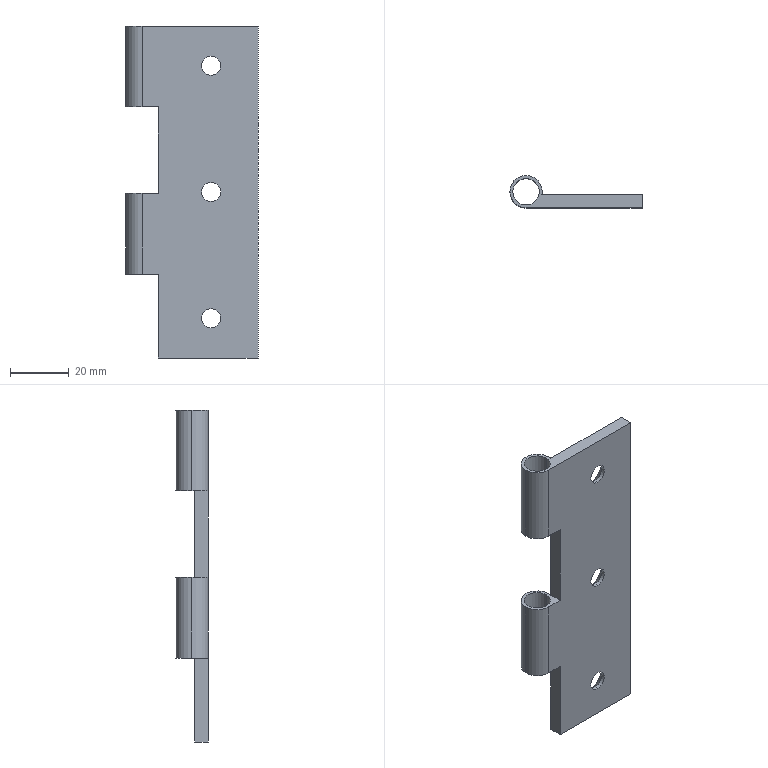Part | SolidWorks | features BaseBody 1 | 1 solid | 32 faces | box 45 x 11 x 113 mm | volume 18493 mm3 | cylinder 16 | plane 10 | cone 6 | commonest cylinder face diameters 6.5 x6 11 x6 9 x4
STEP:
#1=CARTESIAN_POINT('',(23.5,0.,3.25));
#2=VERTEX_POINT('',#1);
#3=CARTESIAN_POINT('',(23.5,0.,-3.25));
#4=VERTEX_POINT('',#3);
#5=CARTESIAN_POINT('',(23.5,0.,0.));
#6=DIRECTION('',(0.,-1.,0.));
#7=DIRECTION('',(0.,0.,1.));
#8=AXIS2_PLACEMENT_3D('',#5,#6,#7);
#9=CIRCLE('',#8,3.25);
#10=EDGE_CURVE('',#2,#4,#9,.T.);
#11=ORIENTED_EDGE('',*,*,#10,.T.);
#12=CARTESIAN_POINT('',(23.5,1.25,-3.25));
#13=VERTEX_POINT('',#12);
#14=CARTESIAN_POINT('',(23.5,0.,-3.25));
#15=DIRECTION('',(0.,1.,0.));
#16=VECTOR('',#15,1000.);
#17=LINE('',#14,#16);
#18=EDGE_CURVE('',#4,#13,#17,.T.);
#19=ORIENTED_EDGE('',*,*,#18,.T.);
#20=CARTESIAN_POINT('',(23.5,1.25,3.25));
#21=VERTEX_POINT('',#20);
#22=CARTESIAN_POINT('',(23.5,1.25,0.));
#23=DIRECTION('',(0.,-1.,0.));
#24=DIRECTION('',(0.,0.,1.));
#25=AXIS2_PLACEMENT_3D('',#22,#23,#24);
#26=CIRCLE('',#25,3.25);
#27=EDGE_CURVE('',#21,#13,#26,.T.);
#28=ORIENTED_EDGE('',*,*,#27,.F.);
#29=CARTESIAN_POINT('',(23.5,0.,3.25));
#30=DIRECTION('',(0.,1.,0.));
#31=VECTOR('',#30,1000.);
#32=LINE('',#29,#31);
#33=EDGE_CURVE('',#2,#21,#32,.T.);
#34=ORIENTED_EDGE('',*,*,#33,.F.);
#35=EDGE_LOOP('',(#11,#19,#28,#34));
#36=FACE_OUTER_BOUND('',#35,.T.);
#37=CARTESIAN_POINT('',(23.5,0.,0.));
#38=DIRECTION('',(0.,1.,0.));
#39=DIRECTION('',(0.,0.,1.));
#40=AXIS2_PLACEMENT_3D('',#37,#38,#39);
#41=CYLINDRICAL_SURFACE('',#40,3.25);
#42=ADVANCED_FACE('',(#36),#41,.F.);
#43=CARTESIAN_POINT('',(23.5,0.,46.25));
#44=VERTEX_POINT('',#43);
#45=CARTESIAN_POINT('',(23.5,0.,39.75));
#46=VERTEX_POINT('',#45);
#47=CARTESIAN_POINT('',(23.5,0.,43.));
#48=DIRECTION('',(0.,-1.,0.));
#49=DIRECTION('',(0.,0.,1.));
#50=AXIS2_PLACEMENT_3D('',#47,#48,#49);
#51=CIRCLE('',#50,3.25);
#52=EDGE_CURVE('',#44,#46,#51,.T.);
#53=ORIENTED_EDGE('',*,*,#52,.T.);
#54=CARTESIAN_POINT('',(23.5,1.25,39.75));
#55=VERTEX_POINT('',#54);
#56=CARTESIAN_POINT('',(23.5,0.,39.75));
#57=DIRECTION('',(0.,1.,0.));
#58=VECTOR('',#57,1000.);
#59=LINE('',#56,#58);
#60=EDGE_CURVE('',#46,#55,#59,.T.);
#61=ORIENTED_EDGE('',*,*,#60,.T.);
#62=CARTESIAN_POINT('',(23.5,1.25,46.25));
#63=VERTEX_POINT('',#62);
#64=CARTESIAN_POINT('',(23.5,1.25,43.));
#65=DIRECTION('',(0.,-1.,0.));
#66=DIRECTION('',(0.,0.,1.));
#67=AXIS2_PLACEMENT_3D('',#64,#65,#66);
#68=CIRCLE('',#67,3.25);
#69=EDGE_CURVE('',#63,#55,#68,.T.);
#70=ORIENTED_EDGE('',*,*,#69,.F.);
#71=CARTESIAN_POINT('',(23.5,0.,46.25));
#72=DIRECTION('',(0.,1.,0.));
#73=VECTOR('',#72,1000.);
#74=LINE('',#71,#73);
#75=EDGE_CURVE('',#44,#63,#74,.T.);
#76=ORIENTED_EDGE('',*,*,#75,.F.);
#77=EDGE_LOOP('',(#53,#61,#70,#76));
#78=FACE_OUTER_BOUND('',#77,.T.);
#79=CARTESIAN_POINT('',(23.5,0.,43.));
#80=DIRECTION('',(0.,1.,0.));
#81=DIRECTION('',(0.,0.,1.));
#82=AXIS2_PLACEMENT_3D('',#79,#80,#81);
#83=CYLINDRICAL_SURFACE('',#82,3.25);
#84=ADVANCED_FACE('',(#78),#83,.F.);
#85=CARTESIAN_POINT('',(23.5,0.,-39.75));
#86=VERTEX_POINT('',#85);
#87=CARTESIAN_POINT('',(23.5,0.,-46.25));
#88=VERTEX_POINT('',#87);
#89=CARTESIAN_POINT('',(23.5,0.,-43.));
#90=DIRECTION('',(0.,-1.,0.));
#91=DIRECTION('',(0.,0.,1.));
#92=AXIS2_PLACEMENT_3D('',#89,#90,#91);
#93=CIRCLE('',#92,3.25);
#94=EDGE_CURVE('',#86,#88,#93,.T.);
#95=ORIENTED_EDGE('',*,*,#94,.T.);
#96=CARTESIAN_POINT('',(23.5,1.25,-46.25));
#97=VERTEX_POINT('',#96);
#98=CARTESIAN_POINT('',(23.5,0.,-46.25));
#99=DIRECTION('',(0.,1.,0.));
#100=VECTOR('',#99,1000.);
#101=LINE('',#98,#100);
#102=EDGE_CURVE('',#88,#97,#101,.T.);
#103=ORIENTED_EDGE('',*,*,#102,.T.);
#104=CARTESIAN_POINT('',(23.5,1.25,-39.75));
#105=VERTEX_POINT('',#104);
#106=CARTESIAN_POINT('',(23.5,1.25,-43.));
#107=DIRECTION('',(0.,-1.,0.));
#108=DIRECTION('',(0.,0.,1.));
#109=AXIS2_PLACEMENT_3D('',#106,#107,#108);
#110=CIRCLE('',#109,3.25);
#111=EDGE_CURVE('',#105,#97,#110,.T.);
#112=ORIENTED_EDGE('',*,*,#111,.F.);
#113=CARTESIAN_POINT('',(23.5,0.,-39.75));
#114=DIRECTION('',(0.,1.,0.));
#115=VECTOR('',#114,1000.);
#116=LINE('',#113,#115);
#117=EDGE_CURVE('',#86,#105,#116,.T.);
#118=ORIENTED_EDGE('',*,*,#117,.F.);
#119=EDGE_LOOP('',(#95,#103,#112,#118));
#120=FACE_OUTER_BOUND('',#119,.T.);
#121=CARTESIAN_POINT('',(23.5,0.,-43.));
#122=DIRECTION('',(0.,1.,0.));
#123=DIRECTION('',(0.,0.,1.));
#124=AXIS2_PLACEMENT_3D('',#121,#122,#123);
#125=CYLINDRICAL_SURFACE('',#124,3.25);
#126=ADVANCED_FACE('',(#120),#125,.F.);
#127=CARTESIAN_POINT('',(5.5,5.5,-28.));
#128=VERTEX_POINT('',#127);
#129=CARTESIAN_POINT('',(-5.5,5.5,-28.));
#130=VERTEX_POINT('',#129);
#131=CARTESIAN_POINT('',(0.,5.5,-28.));
#132=DIRECTION('',(0.,0.,1.));
#133=DIRECTION('',(1.,0.,0.));
#134=AXIS2_PLACEMENT_3D('',#131,#132,#133);
#135=CIRCLE('',#134,5.5);
#136=EDGE_CURVE('',#128,#130,#135,.T.);
#137=ORIENTED_EDGE('',*,*,#136,.T.);
#138=CARTESIAN_POINT('',(-5.5,5.5,-0.5));
#139=VERTEX_POINT('',#138);
#140=CARTESIAN_POINT('',(-5.5,5.5,56.5));
#141=DIRECTION('',(0.,0.,1.));
#142=VECTOR('',#141,1000.);
#143=LINE('',#140,#142);
#144=EDGE_CURVE('',#130,#139,#143,.T.);
#145=ORIENTED_EDGE('',*,*,#144,.T.);
#146=CARTESIAN_POINT('',(5.5,5.5,-0.5));
#147=VERTEX_POINT('',#146);
#148=CARTESIAN_POINT('',(0.,5.5,-0.5));
#149=DIRECTION('',(0.,0.,1.));
#150=DIRECTION('',(1.,0.,0.));
#151=AXIS2_PLACEMENT_3D('',#148,#149,#150);
#152=CIRCLE('',#151,5.5);
#153=EDGE_CURVE('',#147,#139,#152,.T.);
#154=ORIENTED_EDGE('',*,*,#153,.F.);
#155=CARTESIAN_POINT('',(5.5,5.5,56.5));
#156=DIRECTION('',(0.,0.,1.));
#157=VECTOR('',#156,1000.);
#158=LINE('',#155,#157);
#159=EDGE_CURVE('',#128,#147,#158,.T.);
#160=ORIENTED_EDGE('',*,*,#159,.F.);
#161=EDGE_LOOP('',(#137,#145,#154,#160));
#162=FACE_OUTER_BOUND('',#161,.T.);
#163=CARTESIAN_POINT('',(0.,5.5,56.5));
#164=DIRECTION('',(0.,0.,1.));
#165=DIRECTION('',(1.,0.,0.));
#166=AXIS2_PLACEMENT_3D('',#163,#164,#165);
#167=CYLINDRICAL_SURFACE('',#166,5.5);
#168=ADVANCED_FACE('',(#162),#167,.T.);
#169=CARTESIAN_POINT('',(5.408,4.5,-28.));
#170=VERTEX_POINT('',#169);
#171=CARTESIAN_POINT('',(0.,5.5,-28.));
#172=DIRECTION('',(0.,0.,1.));
#173=DIRECTION('',(1.,0.,0.));
#174=AXIS2_PLACEMENT_3D('',#171,#172,#173);
#175=CIRCLE('',#174,5.5);
#176=EDGE_CURVE('',#170,#128,#175,.T.);
#177=ORIENTED_EDGE('',*,*,#176,.T.);
#178=ORIENTED_EDGE('',*,*,#159,.T.);
#179=CARTESIAN_POINT('',(5.408,4.5,-0.5));
#180=VERTEX_POINT('',#179);
#181=CARTESIAN_POINT('',(0.,5.5,-0.5));
#182=DIRECTION('',(0.,0.,1.));
#183=DIRECTION('',(1.,0.,0.));
#184=AXIS2_PLACEMENT_3D('',#181,#182,#183);
#185=CIRCLE('',#184,5.5);
#186=EDGE_CURVE('',#180,#147,#185,.T.);
#187=ORIENTED_EDGE('',*,*,#186,.F.);
#188=CARTESIAN_POINT('',(5.408,4.5,56.5));
#189=DIRECTION('',(0.,0.,-1.));
#190=VECTOR('',#189,1000.);
#191=LINE('',#188,#190);
#192=EDGE_CURVE('',#180,#170,#191,.T.);
#193=ORIENTED_EDGE('',*,*,#192,.T.);
#194=EDGE_LOOP('',(#177,#178,#187,#193));
#195=FACE_OUTER_BOUND('',#194,.T.);
#196=CARTESIAN_POINT('',(0.,5.5,56.5));
#197=DIRECTION('',(0.,0.,1.));
#198=DIRECTION('',(1.,0.,0.));
#199=AXIS2_PLACEMENT_3D('',#196,#197,#198);
#200=CYLINDRICAL_SURFACE('',#199,5.5);
#201=ADVANCED_FACE('',(#195),#200,.T.);
#202=CARTESIAN_POINT('',(5.5,5.5,29.));
#203=VERTEX_POINT('',#202);
#204=CARTESIAN_POINT('',(-5.5,5.5,29.));
#205=VERTEX_POINT('',#204);
#206=CARTESIAN_POINT('',(0.,5.5,29.));
#207=DIRECTION('',(0.,0.,1.));
#208=DIRECTION('',(1.,0.,0.));
#209=AXIS2_PLACEMENT_3D('',#206,#207,#208);
#210=CIRCLE('',#209,5.5);
#211=EDGE_CURVE('',#203,#205,#210,.T.);
#212=ORIENTED_EDGE('',*,*,#211,.T.);
#213=CARTESIAN_POINT('',(-5.5,5.5,56.5));
#214=VERTEX_POINT('',#213);
#215=CARTESIAN_POINT('',(-5.5,5.5,56.5));
#216=DIRECTION('',(0.,0.,1.));
#217=VECTOR('',#216,1000.);
#218=LINE('',#215,#217);
#219=EDGE_CURVE('',#205,#214,#218,.T.);
#220=ORIENTED_EDGE('',*,*,#219,.T.);
#221=CARTESIAN_POINT('',(5.5,5.5,56.5));
#222=VERTEX_POINT('',#221);
#223=CARTESIAN_POINT('',(0.,5.5,56.5));
#224=DIRECTION('',(0.,0.,1.));
#225=DIRECTION('',(1.,0.,0.));
#226=AXIS2_PLACEMENT_3D('',#223,#224,#225);
#227=CIRCLE('',#226,5.5);
#228=EDGE_CURVE('',#222,#214,#227,.T.);
#229=ORIENTED_EDGE('',*,*,#228,.F.);
#230=CARTESIAN_POINT('',(5.5,5.5,56.5));
#231=DIRECTION('',(0.,0.,1.));
#232=VECTOR('',#231,1000.);
#233=LINE('',#230,#232);
#234=EDGE_CURVE('',#203,#222,#233,.T.);
#235=ORIENTED_EDGE('',*,*,#234,.F.);
#236=EDGE_LOOP('',(#212,#220,#229,#235));
#237=FACE_OUTER_BOUND('',#236,.T.);
#238=CARTESIAN_POINT('',(0.,5.5,56.5));
#239=DIRECTION('',(0.,0.,1.));
#240=DIRECTION('',(1.,0.,0.));
#241=AXIS2_PLACEMENT_3D('',#238,#239,#240);
#242=CYLINDRICAL_SURFACE('',#241,5.5);
#243=ADVANCED_FACE('',(#237),#242,.T.);
#244=CARTESIAN_POINT('',(5.408,4.5,29.));
#245=VERTEX_POINT('',#244);
#246=CARTESIAN_POINT('',(0.,5.5,29.));
#247=DIRECTION('',(0.,0.,1.));
#248=DIRECTION('',(1.,0.,0.));
#249=AXIS2_PLACEMENT_3D('',#246,#247,#248);
#250=CIRCLE('',#249,5.5);
#251=EDGE_CURVE('',#245,#203,#250,.T.);
#252=ORIENTED_EDGE('',*,*,#251,.T.);
#253=ORIENTED_EDGE('',*,*,#234,.T.);
#254=CARTESIAN_POINT('',(5.408,4.5,56.5));
#255=VERTEX_POINT('',#254);
#256=CARTESIAN_POINT('',(0.,5.5,56.5));
#257=DIRECTION('',(0.,0.,1.));
#258=DIRECTION('',(1.,0.,0.));
#259=AXIS2_PLACEMENT_3D('',#256,#257,#258);
#260=CIRCLE('',#259,5.5);
#261=EDGE_CURVE('',#255,#222,#260,.T.);
#262=ORIENTED_EDGE('',*,*,#261,.F.);
#263=CARTESIAN_POINT('',(5.408,4.5,56.5));
#264=DIRECTION('',(0.,0.,-1.));
#265=VECTOR('',#264,1000.);
#266=LINE('',#263,#265);
#267=EDGE_CURVE('',#255,#245,#266,.T.);
#268=ORIENTED_EDGE('',*,*,#267,.T.);
#269=EDGE_LOOP('',(#252,#253,#262,#268));
#270=FACE_OUTER_BOUND('',#269,.T.);
#271=CARTESIAN_POINT('',(0.,5.5,56.5));
#272=DIRECTION('',(0.,0.,1.));
#273=DIRECTION('',(1.,0.,0.));
#274=AXIS2_PLACEMENT_3D('',#271,#272,#273);
#275=CYLINDRICAL_SURFACE('',#274,5.5);
#276=ADVANCED_FACE('',(#270),#275,.T.);
#277=ORIENTED_EDGE('',*,*,#27,.T.);
#278=CARTESIAN_POINT('',(23.5,4.5,-6.5));
#279=VERTEX_POINT('',#278);
#280=CARTESIAN_POINT('',(23.5,4.5,-6.5));
#281=DIRECTION('',(0.,0.7071,-0.7071));
#282=VECTOR('',#281,1000.);
#283=LINE('',#280,#282);
#284=EDGE_CURVE('',#13,#279,#283,.T.);
#285=ORIENTED_EDGE('',*,*,#284,.T.);
#286=CARTESIAN_POINT('',(23.5,4.5,6.5));
#287=VERTEX_POINT('',#286);
#288=CARTESIAN_POINT('',(23.5,4.5,0.));
#289=DIRECTION('',(0.,-1.,0.));
#290=DIRECTION('',(0.,0.,1.));
#291=AXIS2_PLACEMENT_3D('',#288,#289,#290);
#292=CIRCLE('',#291,6.5);
#293=EDGE_CURVE('',#287,#279,#292,.T.);
#294=ORIENTED_EDGE('',*,*,#293,.F.);
#295=CARTESIAN_POINT('',(23.5,4.5,6.5));
#296=DIRECTION('',(0.,0.7071,0.7071));
#297=VECTOR('',#296,1000.);
#298=LINE('',#295,#297);
#299=EDGE_CURVE('',#21,#287,#298,.T.);
#300=ORIENTED_EDGE('',*,*,#299,.F.);
#301=EDGE_LOOP('',(#277,#285,#294,#300));
#302=FACE_OUTER_BOUND('',#301,.T.);
#303=CARTESIAN_POINT('',(23.5,4.5,0.));
#304=DIRECTION('',(0.,1.,0.));
#305=DIRECTION('',(0.,0.,1.));
#306=AXIS2_PLACEMENT_3D('',#303,#304,#305);
#307=CONICAL_SURFACE('',#306,6.5,0.7854);
#308=ADVANCED_FACE('',(#302),#307,.F.);
#309=ORIENTED_EDGE('',*,*,#69,.T.);
#310=CARTESIAN_POINT('',(23.5,4.5,36.5));
#311=VERTEX_POINT('',#310);
#312=CARTESIAN_POINT('',(23.5,4.5,36.5));
#313=DIRECTION('',(0.,0.7071,-0.7071));
#314=VECTOR('',#313,1000.);
#315=LINE('',#312,#314);
#316=EDGE_CURVE('',#55,#311,#315,.T.);
#317=ORIENTED_EDGE('',*,*,#316,.T.);
#318=CARTESIAN_POINT('',(23.5,4.5,49.5));
#319=VERTEX_POINT('',#318);
#320=CARTESIAN_POINT('',(23.5,4.5,43.));
#321=DIRECTION('',(0.,-1.,0.));
#322=DIRECTION('',(0.,0.,1.));
#323=AXIS2_PLACEMENT_3D('',#320,#321,#322);
#324=CIRCLE('',#323,6.5);
#325=EDGE_CURVE('',#319,#311,#324,.T.);
#326=ORIENTED_EDGE('',*,*,#325,.F.);
#327=CARTESIAN_POINT('',(23.5,4.5,49.5));
#328=DIRECTION('',(0.,0.7071,0.7071));
#329=VECTOR('',#328,1000.);
#330=LINE('',#327,#329);
#331=EDGE_CURVE('',#63,#319,#330,.T.);
#332=ORIENTED_EDGE('',*,*,#331,.F.);
#333=EDGE_LOOP('',(#309,#317,#326,#332));
#334=FACE_OUTER_BOUND('',#333,.T.);
#335=CARTESIAN_POINT('',(23.5,4.5,43.));
#336=DIRECTION('',(0.,1.,0.));
#337=DIRECTION('',(0.,0.,1.));
#338=AXIS2_PLACEMENT_3D('',#335,#336,#337);
#339=CONICAL_SURFACE('',#338,6.5,0.7854);
#340=ADVANCED_FACE('',(#334),#339,.F.);
#341=ORIENTED_EDGE('',*,*,#111,.T.);
#342=CARTESIAN_POINT('',(23.5,4.5,-49.5));
#343=VERTEX_POINT('',#342);
#344=CARTESIAN_POINT('',(23.5,4.5,-49.5));
#345=DIRECTION('',(0.,0.7071,-0.7071));
#346=VECTOR('',#345,1000.);
#347=LINE('',#344,#346);
#348=EDGE_CURVE('',#97,#343,#347,.T.);
#349=ORIENTED_EDGE('',*,*,#348,.T.);
#350=CARTESIAN_POINT('',(23.5,4.5,-36.5));
#351=VERTEX_POINT('',#350);
#352=CARTESIAN_POINT('',(23.5,4.5,-43.));
#353=DIRECTION('',(0.,-1.,0.));
#354=DIRECTION('',(0.,0.,1.));
#355=AXIS2_PLACEMENT_3D('',#352,#353,#354);
#356=CIRCLE('',#355,6.5);
#357=EDGE_CURVE('',#351,#343,#356,.T.);
#358=ORIENTED_EDGE('',*,*,#357,.F.);
#359=CARTESIAN_POINT('',(23.5,4.5,-36.5));
#360=DIRECTION('',(0.,0.7071,0.7071));
#361=VECTOR('',#360,1000.);
#362=LINE('',#359,#361);
#363=EDGE_CURVE('',#105,#351,#362,.T.);
#364=ORIENTED_EDGE('',*,*,#363,.F.);
#365=EDGE_LOOP('',(#341,#349,#358,#364));
#366=FACE_OUTER_BOUND('',#365,.T.);
#367=CARTESIAN_POINT('',(23.5,4.5,-43.));
#368=DIRECTION('',(0.,1.,0.));
#369=DIRECTION('',(0.,0.,1.));
#370=AXIS2_PLACEMENT_3D('',#367,#368,#369);
#371=CONICAL_SURFACE('',#370,6.5,0.7854);
#372=ADVANCED_FACE('',(#366),#371,.F.);
#373=CARTESIAN_POINT('',(-4.5,5.5,-28.));
#374=VERTEX_POINT('',#373);
#375=CARTESIAN_POINT('',(4.5,5.5,-28.));
#376=VERTEX_POINT('',#375);
#377=CARTESIAN_POINT('',(0.,5.5,-28.));
#378=DIRECTION('',(0.,0.,1.));
#379=DIRECTION('',(1.,0.,0.));
#380=AXIS2_PLACEMENT_3D('',#377,#378,#379);
#381=CIRCLE('',#380,4.5);
#382=EDGE_CURVE('',#374,#376,#381,.T.);
#383=ORIENTED_EDGE('',*,*,#382,.F.);
#384=CARTESIAN_POINT('',(-4.5,5.5,-0.5));
#385=VERTEX_POINT('',#384);
#386=CARTESIAN_POINT('',(-4.5,5.5,56.5));
#387=DIRECTION('',(0.,0.,1.));
#388=VECTOR('',#387,1000.);
#389=LINE('',#386,#388);
#390=EDGE_CURVE('',#374,#385,#389,.T.);
#391=ORIENTED_EDGE('',*,*,#390,.T.);
#392=CARTESIAN_POINT('',(4.5,5.5,-0.5));
#393=VERTEX_POINT('',#392);
#394=CARTESIAN_POINT('',(0.,5.5,-0.5));
#395=DIRECTION('',(0.,0.,-1.));
#396=DIRECTION('',(1.,0.,0.));
#397=AXIS2_PLACEMENT_3D('',#394,#395,#396);
#398=CIRCLE('',#397,4.5);
#399=EDGE_CURVE('',#393,#385,#398,.T.);
#400=ORIENTED_EDGE('',*,*,#399,.F.);
#401=CARTESIAN_POINT('',(4.5,5.5,56.5));
#402=DIRECTION('',(0.,0.,1.));
#403=VECTOR('',#402,1000.);
#404=LINE('',#401,#403);
#405=EDGE_CURVE('',#376,#393,#404,.T.);
#406=ORIENTED_EDGE('',*,*,#405,.F.);
#407=EDGE_LOOP('',(#383,#391,#400,#406));
#408=FACE_OUTER_BOUND('',#407,.T.);
#409=CARTESIAN_POINT('',(0.,5.5,56.5));
#410=DIRECTION('',(0.,0.,1.));
#411=DIRECTION('',(1.,0.,0.));
#412=AXIS2_PLACEMENT_3D('',#409,#410,#411);
#413=CYLINDRICAL_SURFACE('',#412,4.5);
#414=ADVANCED_FACE('',(#408),#413,.F.);
#415=CARTESIAN_POINT('',(-4.5,5.5,29.));
#416=VERTEX_POINT('',#415);
#417=CARTESIAN_POINT('',(4.5,5.5,29.));
#418=VERTEX_POINT('',#417);
#419=CARTESIAN_POINT('',(0.,5.5,29.));
#420=DIRECTION('',(0.,0.,1.));
#421=DIRECTION('',(1.,0.,0.));
#422=AXIS2_PLACEMENT_3D('',#419,#420,#421);
#423=CIRCLE('',#422,4.5);
#424=EDGE_CURVE('',#416,#418,#423,.T.);
#425=ORIENTED_EDGE('',*,*,#424,.F.);
#426=CARTESIAN_POINT('',(-4.5,5.5,56.5));
#427=VERTEX_POINT('',#426);
#428=CARTESIAN_POINT('',(-4.5,5.5,56.5));
#429=DIRECTION('',(0.,0.,1.));
#430=VECTOR('',#429,1000.);
#431=LINE('',#428,#430);
#432=EDGE_CURVE('',#416,#427,#431,.T.);
#433=ORIENTED_EDGE('',*,*,#432,.T.);
#434=CARTESIAN_POINT('',(4.5,5.5,56.5));
#435=VERTEX_POINT('',#434);
#436=CARTESIAN_POINT('',(0.,5.5,56.5));
#437=DIRECTION('',(0.,0.,-1.));
#438=DIRECTION('',(1.,0.,0.));
#439=AXIS2_PLACEMENT_3D('',#436,#437,#438);
#440=CIRCLE('',#439,4.5);
#441=EDGE_CURVE('',#435,#427,#440,.T.);
#442=ORIENTED_EDGE('',*,*,#441,.F.);
#443=CARTESIAN_POINT('',(4.5,5.5,56.5));
#444=DIRECTION('',(0.,0.,1.));
#445=VECTOR('',#444,1000.);
#446=LINE('',#443,#445);
#447=EDGE_CURVE('',#418,#435,#446,.T.);
#448=ORIENTED_EDGE('',*,*,#447,.F.);
#449=EDGE_LOOP('',(#425,#433,#442,#448));
#450=FACE_OUTER_BOUND('',#449,.T.);
#451=CARTESIAN_POINT('',(0.,5.5,56.5));
#452=DIRECTION('',(0.,0.,1.));
#453=DIRECTION('',(1.,0.,0.));
#454=AXIS2_PLACEMENT_3D('',#451,#452,#453);
#455=CYLINDRICAL_SURFACE('',#454,4.5);
#456=ADVANCED_FACE('',(#450),#455,.F.);
#457=ORIENTED_EDGE('',*,*,#10,.F.);
#458=CARTESIAN_POINT('',(23.5,0.,0.));
#459=DIRECTION('',(0.,-1.,0.));
#460=DIRECTION('',(0.,0.,1.));
#461=AXIS2_PLACEMENT_3D('',#458,#459,#460);
#462=CIRCLE('',#461,3.25);
#463=EDGE_CURVE('',#4,#2,#462,.T.);
#464=ORIENTED_EDGE('',*,*,#463,.F.);
#465=EDGE_LOOP('',(#457,#464));
#466=FACE_BOUND('',#465,.T.);
#467=ORIENTED_EDGE('',*,*,#52,.F.);
#468=CARTESIAN_POINT('',(23.5,0.,43.));
#469=DIRECTION('',(0.,-1.,0.));
#470=DIRECTION('',(0.,0.,1.));
#471=AXIS2_PLACEMENT_3D('',#468,#469,#470);
#472=CIRCLE('',#471,3.25);
#473=EDGE_CURVE('',#46,#44,#472,.T.);
#474=ORIENTED_EDGE('',*,*,#473,.F.);
#475=EDGE_LOOP('',(#467,#474));
#476=FACE_BOUND('',#475,.T.);
#477=ORIENTED_EDGE('',*,*,#94,.F.);
#478=CARTESIAN_POINT('',(23.5,0.,-43.));
#479=DIRECTION('',(0.,-1.,0.));
#480=DIRECTION('',(0.,0.,1.));
#481=AXIS2_PLACEMENT_3D('',#478,#479,#480);
#482=CIRCLE('',#481,3.25);
#483=EDGE_CURVE('',#88,#86,#482,.T.);
#484=ORIENTED_EDGE('',*,*,#483,.F.);
#485=EDGE_LOOP('',(#477,#484));
#486=FACE_BOUND('',#485,.T.);
#487=CARTESIAN_POINT('',(0.,0.,-0.5));
#488=VERTEX_POINT('',#487);
#489=CARTESIAN_POINT('',(5.5,0.,-0.5));
#490=VERTEX_POINT('',#489);
#491=CARTESIAN_POINT('',(0.,0.,-0.5));
#492=DIRECTION('',(1.,0.,0.));
#493=VECTOR('',#492,1000.);
#494=LINE('',#491,#493);
#495=EDGE_CURVE('',#488,#490,#494,.T.);
#496=ORIENTED_EDGE('',*,*,#495,.F.);
#497=CARTESIAN_POINT('',(0.,0.,-28.));
#498=VERTEX_POINT('',#497);
#499=CARTESIAN_POINT('',(0.,0.,56.5));
#500=DIRECTION('',(0.,0.,1.));
#501=VECTOR('',#500,1000.);
#502=LINE('',#499,#501);
#503=EDGE_CURVE('',#498,#488,#502,.T.);
#504=ORIENTED_EDGE('',*,*,#503,.F.);
#505=CARTESIAN_POINT('',(5.5,0.,-28.));
#506=VERTEX_POINT('',#505);
#507=CARTESIAN_POINT('',(0.,0.,-28.));
#508=DIRECTION('',(-1.,0.,0.));
#509=VECTOR('',#508,1000.);
#510=LINE('',#507,#509);
#511=EDGE_CURVE('',#506,#498,#510,.T.);
#512=ORIENTED_EDGE('',*,*,#511,.F.);
#513=CARTESIAN_POINT('',(5.5,0.,-56.5));
#514=VERTEX_POINT('',#513);
#515=CARTESIAN_POINT('',(5.5,0.,56.5));
#516=DIRECTION('',(0.,0.,1.));
#517=VECTOR('',#516,1000.);
#518=LINE('',#515,#517);
#519=EDGE_CURVE('',#514,#506,#518,.T.);
#520=ORIENTED_EDGE('',*,*,#519,.F.);
#521=CARTESIAN_POINT('',(39.5,0.,-56.5));
#522=VERTEX_POINT('',#521);
#523=CARTESIAN_POINT('',(0.,0.,-56.5));
#524=DIRECTION('',(-1.,0.,0.));
#525=VECTOR('',#524,1000.);
#526=LINE('',#523,#525);
#527=EDGE_CURVE('',#522,#514,#526,.T.);
#528=ORIENTED_EDGE('',*,*,#527,.F.);
#529=CARTESIAN_POINT('',(39.5,0.,56.5));
#530=VERTEX_POINT('',#529);
#531=CARTESIAN_POINT('',(39.5,0.,56.5));
#532=DIRECTION('',(0.,0.,-1.));
#533=VECTOR('',#532,1000.);
#534=LINE('',#531,#533);
#535=EDGE_CURVE('',#530,#522,#534,.T.);
#536=ORIENTED_EDGE('',*,*,#535,.F.);
#537=CARTESIAN_POINT('',(0.,0.,56.5));
#538=VERTEX_POINT('',#537);
#539=CARTESIAN_POINT('',(0.,0.,56.5));
#540=DIRECTION('',(1.,0.,0.));
#541=VECTOR('',#540,1000.);
#542=LINE('',#539,#541);
#543=EDGE_CURVE('',#538,#530,#542,.T.);
#544=ORIENTED_EDGE('',*,*,#543,.F.);
#545=CARTESIAN_POINT('',(0.,0.,29.));
#546=VERTEX_POINT('',#545);
#547=CARTESIAN_POINT('',(0.,0.,56.5));
#548=DIRECTION('',(0.,0.,1.));
#549=VECTOR('',#548,1000.);
#550=LINE('',#547,#549);
#551=EDGE_CURVE('',#546,#538,#550,.T.);
#552=ORIENTED_EDGE('',*,*,#551,.F.);
#553=CARTESIAN_POINT('',(5.5,0.,29.));
#554=VERTEX_POINT('',#553);
#555=CARTESIAN_POINT('',(0.,0.,29.));
#556=DIRECTION('',(-1.,0.,0.));
#557=VECTOR('',#556,1000.);
#558=LINE('',#555,#557);
#559=EDGE_CURVE('',#554,#546,#558,.T.);
#560=ORIENTED_EDGE('',*,*,#559,.F.);
#561=CARTESIAN_POINT('',(5.5,0.,56.5));
#562=DIRECTION('',(0.,0.,1.));
#563=VECTOR('',#562,1000.);
#564=LINE('',#561,#563);
#565=EDGE_CURVE('',#490,#554,#564,.T.);
#566=ORIENTED_EDGE('',*,*,#565,.F.);
#567=EDGE_LOOP('',(#496,#504,#512,#520,#528,#536,#544,#552,#560,#566));
#568=FACE_OUTER_BOUND('',#567,.T.);
#569=CARTESIAN_POINT('',(0.,0.,56.5));
#570=DIRECTION('',(0.,1.,0.));
#571=DIRECTION('',(0.,0.,1.));
#572=AXIS2_PLACEMENT_3D('',#569,#570,#571);
#573=PLANE('',#572);
#574=ADVANCED_FACE('',(#466,#476,#486,#568),#573,.F.);
#575=ORIENTED_EDGE('',*,*,#18,.F.);
#576=ORIENTED_EDGE('',*,*,#463,.T.);
#577=ORIENTED_EDGE('',*,*,#33,.T.);
#578=CARTESIAN_POINT('',(23.5,1.25,0.));
#579=DIRECTION('',(0.,-1.,0.));
#580=DIRECTION('',(0.,0.,1.));
#581=AXIS2_PLACEMENT_3D('',#578,#579,#580);
#582=CIRCLE('',#581,3.25);
#583=EDGE_CURVE('',#13,#21,#582,.T.);
#584=ORIENTED_EDGE('',*,*,#583,.F.);
#585=EDGE_LOOP('',(#575,#576,#577,#584));
#586=FACE_OUTER_BOUND('',#585,.T.);
#587=CARTESIAN_POINT('',(23.5,0.,0.));
#588=DIRECTION('',(0.,1.,0.));
#589=DIRECTION('',(0.,0.,1.));
#590=AXIS2_PLACEMENT_3D('',#587,#588,#589);
#591=CYLINDRICAL_SURFACE('',#590,3.25);
#592=ADVANCED_FACE('',(#586),#591,.F.);
#593=ORIENTED_EDGE('',*,*,#60,.F.);
#594=ORIENTED_EDGE('',*,*,#473,.T.);
#595=ORIENTED_EDGE('',*,*,#75,.T.);
#596=CARTESIAN_POINT('',(23.5,1.25,43.));
#597=DIRECTION('',(0.,-1.,0.));
#598=DIRECTION('',(0.,0.,1.));
#599=AXIS2_PLACEMENT_3D('',#596,#597,#598);
#600=CIRCLE('',#599,3.25);
#601=EDGE_CURVE('',#55,#63,#600,.T.);
#602=ORIENTED_EDGE('',*,*,#601,.F.);
#603=EDGE_LOOP('',(#593,#594,#595,#602));
#604=FACE_OUTER_BOUND('',#603,.T.);
#605=CARTESIAN_POINT('',(23.5,0.,43.));
#606=DIRECTION('',(0.,1.,0.));
#607=DIRECTION('',(0.,0.,1.));
#608=AXIS2_PLACEMENT_3D('',#605,#606,#607);
#609=CYLINDRICAL_SURFACE('',#608,3.25);
#610=ADVANCED_FACE('',(#604),#609,.F.);
#611=ORIENTED_EDGE('',*,*,#102,.F.);
#612=ORIENTED_EDGE('',*,*,#483,.T.);
#613=ORIENTED_EDGE('',*,*,#117,.T.);
#614=CARTESIAN_POINT('',(23.5,1.25,-43.));
#615=DIRECTION('',(0.,-1.,0.));
#616=DIRECTION('',(0.,0.,1.));
#617=AXIS2_PLACEMENT_3D('',#614,#615,#616);
#618=CIRCLE('',#617,3.25);
#619=EDGE_CURVE('',#97,#105,#618,.T.);
#620=ORIENTED_EDGE('',*,*,#619,.F.);
#621=EDGE_LOOP('',(#611,#612,#613,#620));
#622=FACE_OUTER_BOUND('',#621,.T.);
#623=CARTESIAN_POINT('',(23.5,0.,-43.));
#624=DIRECTION('',(0.,1.,0.));
#625=DIRECTION('',(0.,0.,1.));
#626=AXIS2_PLACEMENT_3D('',#623,#624,#625);
#627=CYLINDRICAL_SURFACE('',#626,3.25);
#628=ADVANCED_FACE('',(#622),#627,.F.);
#629=CARTESIAN_POINT('',(5.5,4.5,29.));
#630=VERTEX_POINT('',#629);
#631=CARTESIAN_POINT('',(5.5,4.5,-0.5));
#632=VERTEX_POINT('',#631);
#633=CARTESIAN_POINT('',(5.5,4.5,29.));
#634=DIRECTION('',(0.,0.,-1.));
#635=VECTOR('',#634,1000.);
#636=LINE('',#633,#635);
#637=EDGE_CURVE('',#630,#632,#636,.T.);
#638=ORIENTED_EDGE('',*,*,#637,.T.);
#639=CARTESIAN_POINT('',(5.5,11.,-0.5));
#640=DIRECTION('',(0.,-1.,0.));
#641=VECTOR('',#640,1000.);
#642=LINE('',#639,#641);
#643=EDGE_CURVE('',#632,#490,#642,.T.);
#644=ORIENTED_EDGE('',*,*,#643,.T.);
#645=ORIENTED_EDGE('',*,*,#565,.T.);
#646=CARTESIAN_POINT('',(5.5,11.,29.));
#647=DIRECTION('',(0.,1.,0.));
#648=VECTOR('',#647,1000.);
#649=LINE('',#646,#648);
#650=EDGE_CURVE('',#554,#630,#649,.T.);
#651=ORIENTED_EDGE('',*,*,#650,.T.);
#652=EDGE_LOOP('',(#638,#644,#645,#651));
#653=FACE_OUTER_BOUND('',#652,.T.);
#654=CARTESIAN_POINT('',(5.5,11.,29.));
#655=DIRECTION('',(-1.,0.,0.));
#656=DIRECTION('',(0.,0.,1.));
#657=AXIS2_PLACEMENT_3D('',#654,#655,#656);
#658=PLANE('',#657);
#659=ADVANCED_FACE('',(#653),#658,.T.);
#660=ORIENTED_EDGE('',*,*,#399,.T.);
#661=CARTESIAN_POINT('',(0.,5.5,-0.5));
#662=DIRECTION('',(0.,0.,-1.));
#663=DIRECTION('',(1.,0.,0.));
#664=AXIS2_PLACEMENT_3D('',#661,#662,#663);
#665=CIRCLE('',#664,4.5);
#666=EDGE_CURVE('',#385,#393,#665,.T.);
#667=ORIENTED_EDGE('',*,*,#666,.T.);
#668=EDGE_LOOP('',(#660,#667));
#669=FACE_BOUND('',#668,.T.);
#670=CARTESIAN_POINT('',(5.5,4.5,-0.5));
#671=DIRECTION('',(-1.,0.,0.));
#672=VECTOR('',#671,1000.);
#673=LINE('',#670,#672);
#674=EDGE_CURVE('',#632,#180,#673,.T.);
#675=ORIENTED_EDGE('',*,*,#674,.T.);
#676=ORIENTED_EDGE('',*,*,#186,.T.);
#677=ORIENTED_EDGE('',*,*,#153,.T.);
#678=CARTESIAN_POINT('',(0.,5.5,-0.5));
#679=DIRECTION('',(0.,0.,1.));
#680=DIRECTION('',(1.,0.,0.));
#681=AXIS2_PLACEMENT_3D('',#678,#679,#680);
#682=CIRCLE('',#681,5.5);
#683=EDGE_CURVE('',#139,#488,#682,.T.);
#684=ORIENTED_EDGE('',*,*,#683,.T.);
#685=ORIENTED_EDGE('',*,*,#495,.T.);
#686=ORIENTED_EDGE('',*,*,#643,.F.);
#687=EDGE_LOOP('',(#675,#676,#677,#684,#685,#686));
#688=FACE_OUTER_BOUND('',#687,.T.);
#689=CARTESIAN_POINT('',(5.5,11.,-0.5));
#690=DIRECTION('',(0.,0.,1.));
#691=DIRECTION('',(1.,0.,0.));
#692=AXIS2_PLACEMENT_3D('',#689,#690,#691);
#693=PLANE('',#692);
#694=ADVANCED_FACE('',(#669,#688),#693,.T.);
#695=ORIENTED_EDGE('',*,*,#144,.F.);
#696=CARTESIAN_POINT('',(0.,5.5,-28.));
#697=DIRECTION('',(0.,0.,1.));
#698=DIRECTION('',(1.,0.,0.));
#699=AXIS2_PLACEMENT_3D('',#696,#697,#698);
#700=CIRCLE('',#699,5.5);
#701=EDGE_CURVE('',#130,#498,#700,.T.);
#702=ORIENTED_EDGE('',*,*,#701,.T.);
#703=ORIENTED_EDGE('',*,*,#503,.T.);
#704=ORIENTED_EDGE('',*,*,#683,.F.);
#705=EDGE_LOOP('',(#695,#702,#703,#704));
#706=FACE_OUTER_BOUND('',#705,.T.);
#707=CARTESIAN_POINT('',(0.,5.5,56.5));
#708=DIRECTION('',(0.,0.,1.));
#709=DIRECTION('',(1.,0.,0.));
#710=AXIS2_PLACEMENT_3D('',#707,#708,#709);
#711=CYLINDRICAL_SURFACE('',#710,5.5);
#712=ADVANCED_FACE('',(#706),#711,.T.);
#713=CARTESIAN_POINT('',(0.,5.5,-28.));
#714=DIRECTION('',(0.,0.,1.));
#715=DIRECTION('',(1.,0.,0.));
#716=AXIS2_PLACEMENT_3D('',#713,#714,#715);
#717=CIRCLE('',#716,4.5);
#718=EDGE_CURVE('',#376,#374,#717,.T.);
#719=ORIENTED_EDGE('',*,*,#718,.T.);
#720=ORIENTED_EDGE('',*,*,#382,.T.);
#721=EDGE_LOOP('',(#719,#720));
#722=FACE_BOUND('',#721,.T.);
#723=CARTESIAN_POINT('',(5.5,4.5,-28.));
#724=VERTEX_POINT('',#723);
#725=CARTESIAN_POINT('',(-5.5,4.5,-28.));
#726=DIRECTION('',(1.,0.,0.));
#727=VECTOR('',#726,1000.);
#728=LINE('',#725,#727);
#729=EDGE_CURVE('',#170,#724,#728,.T.);
#730=ORIENTED_EDGE('',*,*,#729,.T.);
#731=CARTESIAN_POINT('',(5.5,11.,-28.));
#732=DIRECTION('',(0.,-1.,0.));
#733=VECTOR('',#732,1000.);
#734=LINE('',#731,#733);
#735=EDGE_CURVE('',#724,#506,#734,.T.);
#736=ORIENTED_EDGE('',*,*,#735,.T.);
#737=ORIENTED_EDGE('',*,*,#511,.T.);
#738=ORIENTED_EDGE('',*,*,#701,.F.);
#739=ORIENTED_EDGE('',*,*,#136,.F.);
#740=ORIENTED_EDGE('',*,*,#176,.F.);
#741=EDGE_LOOP('',(#730,#736,#737,#738,#739,#740));
#742=FACE_OUTER_BOUND('',#741,.T.);
#743=CARTESIAN_POINT('',(-5.5,11.,-28.));
#744=DIRECTION('',(0.,0.,-1.));
#745=DIRECTION('',(-1.,0.,0.));
#746=AXIS2_PLACEMENT_3D('',#743,#744,#745);
#747=PLANE('',#746);
#748=ADVANCED_FACE('',(#722,#742),#747,.T.);
#749=CARTESIAN_POINT('',(5.5,4.5,-56.5));
#750=VERTEX_POINT('',#749);
#751=CARTESIAN_POINT('',(5.5,4.5,-28.));
#752=DIRECTION('',(0.,0.,-1.));
#753=VECTOR('',#752,1000.);
#754=LINE('',#751,#753);
#755=EDGE_CURVE('',#724,#750,#754,.T.);
#756=ORIENTED_EDGE('',*,*,#755,.T.);
#757=CARTESIAN_POINT('',(5.5,11.,-56.5));
#758=DIRECTION('',(0.,-1.,0.));
#759=VECTOR('',#758,1000.);
#760=LINE('',#757,#759);
#761=EDGE_CURVE('',#750,#514,#760,.T.);
#762=ORIENTED_EDGE('',*,*,#761,.T.);
#763=ORIENTED_EDGE('',*,*,#519,.T.);
#764=ORIENTED_EDGE('',*,*,#735,.F.);
#765=EDGE_LOOP('',(#756,#762,#763,#764));
#766=FACE_OUTER_BOUND('',#765,.T.);
#767=CARTESIAN_POINT('',(5.5,11.,-28.));
#768=DIRECTION('',(-1.,0.,0.));
#769=DIRECTION('',(0.,0.,1.));
#770=AXIS2_PLACEMENT_3D('',#767,#768,#769);
#771=PLANE('',#770);
#772=ADVANCED_FACE('',(#766),#771,.T.);
#773=CARTESIAN_POINT('',(39.5,4.5,-56.5));
#774=VERTEX_POINT('',#773);
#775=CARTESIAN_POINT('',(39.5,5.5,-56.5));
#776=DIRECTION('',(0.,1.,0.));
#777=VECTOR('',#776,1000.);
#778=LINE('',#775,#777);
#779=EDGE_CURVE('',#522,#774,#778,.T.);
#780=ORIENTED_EDGE('',*,*,#779,.F.);
#781=ORIENTED_EDGE('',*,*,#527,.T.);
#782=ORIENTED_EDGE('',*,*,#761,.F.);
#783=CARTESIAN_POINT('',(0.,4.5,-56.5));
#784=DIRECTION('',(-1.,0.,0.));
#785=VECTOR('',#784,1000.);
#786=LINE('',#783,#785);
#787=EDGE_CURVE('',#774,#750,#786,.T.);
#788=ORIENTED_EDGE('',*,*,#787,.F.);
#789=EDGE_LOOP('',(#780,#781,#782,#788));
#790=FACE_OUTER_BOUND('',#789,.T.);
#791=CARTESIAN_POINT('',(0.,5.5,-56.5));
#792=DIRECTION('',(0.,0.,1.));
#793=DIRECTION('',(1.,0.,0.));
#794=AXIS2_PLACEMENT_3D('',#791,#792,#793);
#795=PLANE('',#794);
#796=ADVANCED_FACE('',(#790),#795,.F.);
#797=CARTESIAN_POINT('',(39.5,4.5,56.5));
#798=VERTEX_POINT('',#797);
#799=CARTESIAN_POINT('',(39.5,0.,56.5));
#800=DIRECTION('',(0.,1.,0.));
#801=VECTOR('',#800,1000.);
#802=LINE('',#799,#801);
#803=EDGE_CURVE('',#530,#798,#802,.T.);
#804=ORIENTED_EDGE('',*,*,#803,.F.);
#805=ORIENTED_EDGE('',*,*,#535,.T.);
#806=ORIENTED_EDGE('',*,*,#779,.T.);
#807=CARTESIAN_POINT('',(39.5,4.5,56.5));
#808=DIRECTION('',(0.,0.,-1.));
#809=VECTOR('',#808,1000.);
#810=LINE('',#807,#809);
#811=EDGE_CURVE('',#798,#774,#810,.T.);
#812=ORIENTED_EDGE('',*,*,#811,.F.);
#813=EDGE_LOOP('',(#804,#805,#806,#812));
#814=FACE_OUTER_BOUND('',#813,.T.);
#815=CARTESIAN_POINT('',(39.5,0.,56.5));
#816=DIRECTION('',(-1.,0.,0.));
#817=DIRECTION('',(0.,0.,1.));
#818=AXIS2_PLACEMENT_3D('',#815,#816,#817);
#819=PLANE('',#818);
#820=ADVANCED_FACE('',(#814),#819,.F.);
#821=ORIENTED_EDGE('',*,*,#441,.T.);
#822=CARTESIAN_POINT('',(0.,5.5,56.5));
#823=DIRECTION('',(0.,0.,-1.));
#824=DIRECTION('',(1.,0.,0.));
#825=AXIS2_PLACEMENT_3D('',#822,#823,#824);
#826=CIRCLE('',#825,4.5);
#827=EDGE_CURVE('',#427,#435,#826,.T.);
#828=ORIENTED_EDGE('',*,*,#827,.T.);
#829=EDGE_LOOP('',(#821,#828));
#830=FACE_BOUND('',#829,.T.);
#831=CARTESIAN_POINT('',(0.,4.5,56.5));
#832=DIRECTION('',(-1.,0.,0.));
#833=VECTOR('',#832,1000.);
#834=LINE('',#831,#833);
#835=EDGE_CURVE('',#798,#255,#834,.T.);
#836=ORIENTED_EDGE('',*,*,#835,.T.);
#837=ORIENTED_EDGE('',*,*,#261,.T.);
#838=ORIENTED_EDGE('',*,*,#228,.T.);
#839=CARTESIAN_POINT('',(0.,5.5,56.5));
#840=DIRECTION('',(0.,0.,1.));
#841=DIRECTION('',(1.,0.,0.));
#842=AXIS2_PLACEMENT_3D('',#839,#840,#841);
#843=CIRCLE('',#842,5.5);
#844=EDGE_CURVE('',#214,#538,#843,.T.);
#845=ORIENTED_EDGE('',*,*,#844,.T.);
#846=ORIENTED_EDGE('',*,*,#543,.T.);
#847=ORIENTED_EDGE('',*,*,#803,.T.);
#848=EDGE_LOOP('',(#836,#837,#838,#845,#846,#847));
#849=FACE_OUTER_BOUND('',#848,.T.);
#850=CARTESIAN_POINT('',(0.,5.5,56.5));
#851=DIRECTION('',(0.,0.,1.));
#852=DIRECTION('',(1.,0.,0.));
#853=AXIS2_PLACEMENT_3D('',#850,#851,#852);
#854=PLANE('',#853);
#855=ADVANCED_FACE('',(#830,#849),#854,.T.);
#856=ORIENTED_EDGE('',*,*,#219,.F.);
#857=CARTESIAN_POINT('',(0.,5.5,29.));
#858=DIRECTION('',(0.,0.,1.));
#859=DIRECTION('',(1.,0.,0.));
#860=AXIS2_PLACEMENT_3D('',#857,#858,#859);
#861=CIRCLE('',#860,5.5);
#862=EDGE_CURVE('',#205,#546,#861,.T.);
#863=ORIENTED_EDGE('',*,*,#862,.T.);
#864=ORIENTED_EDGE('',*,*,#551,.T.);
#865=ORIENTED_EDGE('',*,*,#844,.F.);
#866=EDGE_LOOP('',(#856,#863,#864,#865));
#867=FACE_OUTER_BOUND('',#866,.T.);
#868=CARTESIAN_POINT('',(0.,5.5,56.5));
#869=DIRECTION('',(0.,0.,1.));
#870=DIRECTION('',(1.,0.,0.));
#871=AXIS2_PLACEMENT_3D('',#868,#869,#870);
#872=CYLINDRICAL_SURFACE('',#871,5.5);
#873=ADVANCED_FACE('',(#867),#872,.T.);
#874=CARTESIAN_POINT('',(0.,5.5,29.));
#875=DIRECTION('',(0.,0.,1.));
#876=DIRECTION('',(1.,0.,0.));
#877=AXIS2_PLACEMENT_3D('',#874,#875,#876);
#878=CIRCLE('',#877,4.5);
#879=EDGE_CURVE('',#418,#416,#878,.T.);
#880=ORIENTED_EDGE('',*,*,#879,.T.);
#881=ORIENTED_EDGE('',*,*,#424,.T.);
#882=EDGE_LOOP('',(#880,#881));
#883=FACE_BOUND('',#882,.T.);
#884=CARTESIAN_POINT('',(-7.5,4.5,29.));
#885=DIRECTION('',(1.,0.,0.));
#886=VECTOR('',#885,1000.);
#887=LINE('',#884,#886);
#888=EDGE_CURVE('',#245,#630,#887,.T.);
#889=ORIENTED_EDGE('',*,*,#888,.T.);
#890=ORIENTED_EDGE('',*,*,#650,.F.);
#891=ORIENTED_EDGE('',*,*,#559,.T.);
#892=ORIENTED_EDGE('',*,*,#862,.F.);
#893=ORIENTED_EDGE('',*,*,#211,.F.);
#894=ORIENTED_EDGE('',*,*,#251,.F.);
#895=EDGE_LOOP('',(#889,#890,#891,#892,#893,#894));
#896=FACE_OUTER_BOUND('',#895,.T.);
#897=CARTESIAN_POINT('',(-7.5,11.,29.));
#898=DIRECTION('',(0.,0.,-1.));
#899=DIRECTION('',(-1.,0.,0.));
#900=AXIS2_PLACEMENT_3D('',#897,#898,#899);
#901=PLANE('',#900);
#902=ADVANCED_FACE('',(#883,#896),#901,.T.);
#903=ORIENTED_EDGE('',*,*,#284,.F.);
#904=ORIENTED_EDGE('',*,*,#583,.T.);
#905=ORIENTED_EDGE('',*,*,#299,.T.);
#906=CARTESIAN_POINT('',(23.5,4.5,0.));
#907=DIRECTION('',(0.,-1.,0.));
#908=DIRECTION('',(0.,0.,1.));
#909=AXIS2_PLACEMENT_3D('',#906,#907,#908);
#910=CIRCLE('',#909,6.5);
#911=EDGE_CURVE('',#279,#287,#910,.T.);
#912=ORIENTED_EDGE('',*,*,#911,.F.);
#913=EDGE_LOOP('',(#903,#904,#905,#912));
#914=FACE_OUTER_BOUND('',#913,.T.);
#915=CARTESIAN_POINT('',(23.5,4.5,0.));
#916=DIRECTION('',(0.,1.,0.));
#917=DIRECTION('',(0.,0.,1.));
#918=AXIS2_PLACEMENT_3D('',#915,#916,#917);
#919=CONICAL_SURFACE('',#918,6.5,0.7854);
#920=ADVANCED_FACE('',(#914),#919,.F.);
#921=ORIENTED_EDGE('',*,*,#316,.F.);
#922=ORIENTED_EDGE('',*,*,#601,.T.);
#923=ORIENTED_EDGE('',*,*,#331,.T.);
#924=CARTESIAN_POINT('',(23.5,4.5,43.));
#925=DIRECTION('',(0.,-1.,0.));
#926=DIRECTION('',(0.,0.,1.));
#927=AXIS2_PLACEMENT_3D('',#924,#925,#926);
#928=CIRCLE('',#927,6.5);
#929=EDGE_CURVE('',#311,#319,#928,.T.);
#930=ORIENTED_EDGE('',*,*,#929,.F.);
#931=EDGE_LOOP('',(#921,#922,#923,#930));
#932=FACE_OUTER_BOUND('',#931,.T.);
#933=CARTESIAN_POINT('',(23.5,4.5,43.));
#934=DIRECTION('',(0.,1.,0.));
#935=DIRECTION('',(0.,0.,1.));
#936=AXIS2_PLACEMENT_3D('',#933,#934,#935);
#937=CONICAL_SURFACE('',#936,6.5,0.7854);
#938=ADVANCED_FACE('',(#932),#937,.F.);
#939=ORIENTED_EDGE('',*,*,#348,.F.);
#940=ORIENTED_EDGE('',*,*,#619,.T.);
#941=ORIENTED_EDGE('',*,*,#363,.T.);
#942=CARTESIAN_POINT('',(23.5,4.5,-43.));
#943=DIRECTION('',(0.,-1.,0.));
#944=DIRECTION('',(0.,0.,1.));
#945=AXIS2_PLACEMENT_3D('',#942,#943,#944);
#946=CIRCLE('',#945,6.5);
#947=EDGE_CURVE('',#343,#351,#946,.T.);
#948=ORIENTED_EDGE('',*,*,#947,.F.);
#949=EDGE_LOOP('',(#939,#940,#941,#948));
#950=FACE_OUTER_BOUND('',#949,.T.);
#951=CARTESIAN_POINT('',(23.5,4.5,-43.));
#952=DIRECTION('',(0.,1.,0.));
#953=DIRECTION('',(0.,0.,1.));
#954=AXIS2_PLACEMENT_3D('',#951,#952,#953);
#955=CONICAL_SURFACE('',#954,6.5,0.7854);
#956=ADVANCED_FACE('',(#950),#955,.F.);
#957=ORIENTED_EDGE('',*,*,#293,.T.);
#958=ORIENTED_EDGE('',*,*,#911,.T.);
#959=EDGE_LOOP('',(#957,#958));
#960=FACE_BOUND('',#959,.T.);
#961=ORIENTED_EDGE('',*,*,#325,.T.);
#962=ORIENTED_EDGE('',*,*,#929,.T.);
#963=EDGE_LOOP('',(#961,#962));
#964=FACE_BOUND('',#963,.T.);
#965=ORIENTED_EDGE('',*,*,#357,.T.);
#966=ORIENTED_EDGE('',*,*,#947,.T.);
#967=EDGE_LOOP('',(#965,#966));
#968=FACE_BOUND('',#967,.T.);
#969=ORIENTED_EDGE('',*,*,#835,.F.);
#970=ORIENTED_EDGE('',*,*,#811,.T.);
#971=ORIENTED_EDGE('',*,*,#787,.T.);
#972=ORIENTED_EDGE('',*,*,#755,.F.);
#973=ORIENTED_EDGE('',*,*,#729,.F.);
#974=ORIENTED_EDGE('',*,*,#192,.F.);
#975=ORIENTED_EDGE('',*,*,#674,.F.);
#976=ORIENTED_EDGE('',*,*,#637,.F.);
#977=ORIENTED_EDGE('',*,*,#888,.F.);
#978=ORIENTED_EDGE('',*,*,#267,.F.);
#979=EDGE_LOOP('',(#969,#970,#971,#972,#973,#974,#975,#976,#977,#978));
#980=FACE_OUTER_BOUND('',#979,.T.);
#981=CARTESIAN_POINT('',(39.5,4.5,56.5));
#982=DIRECTION('',(0.,-1.,0.));
#983=DIRECTION('',(0.,0.,-1.));
#984=AXIS2_PLACEMENT_3D('',#981,#982,#983);
#985=PLANE('',#984);
#986=ADVANCED_FACE('',(#960,#964,#968,#980),#985,.F.);
#987=ORIENTED_EDGE('',*,*,#390,.F.);
#988=ORIENTED_EDGE('',*,*,#718,.F.);
#989=ORIENTED_EDGE('',*,*,#405,.T.);
#990=ORIENTED_EDGE('',*,*,#666,.F.);
#991=EDGE_LOOP('',(#987,#988,#989,#990));
#992=FACE_OUTER_BOUND('',#991,.T.);
#993=CARTESIAN_POINT('',(0.,5.5,56.5));
#994=DIRECTION('',(0.,0.,1.));
#995=DIRECTION('',(1.,0.,0.));
#996=AXIS2_PLACEMENT_3D('',#993,#994,#995);
#997=CYLINDRICAL_SURFACE('',#996,4.5);
#998=ADVANCED_FACE('',(#992),#997,.F.);
#999=ORIENTED_EDGE('',*,*,#432,.F.);
#1000=ORIENTED_EDGE('',*,*,#879,.F.);
#1001=ORIENTED_EDGE('',*,*,#447,.T.);
#1002=ORIENTED_EDGE('',*,*,#827,.F.);
#1003=EDGE_LOOP('',(#999,#1000,#1001,#1002));
#1004=FACE_OUTER_BOUND('',#1003,.T.);
#1005=CARTESIAN_POINT('',(0.,5.5,56.5));
#1006=DIRECTION('',(0.,0.,1.));
#1007=DIRECTION('',(1.,0.,0.));
#1008=AXIS2_PLACEMENT_3D('',#1005,#1006,#1007);
#1009=CYLINDRICAL_SURFACE('',#1008,4.5);
#1010=ADVANCED_FACE('',(#1004),#1009,.F.);
#1011=CLOSED_SHELL('',(#42,#84,#126,#168,#201,#243,#276,#308,#340,#372,#414,#456,#574,#592,#610,#628,#659,#694,#712,#748,#772,#796,#820,#855,#873,#902,#920,#938,#956,#986,#998,#1010));
#1012=MANIFOLD_SOLID_BREP('',#1011);
#1013=CARTESIAN_POINT('',(0.,0.,0.));
#1014=DIRECTION('',(0.,0.,1.));
#1015=DIRECTION('',(1.,0.,0.));
#1016=AXIS2_PLACEMENT_3D('',#1013,#1014,#1015);
#1017=(LENGTH_UNIT()NAMED_UNIT(*)SI_UNIT(.MILLI.,.METRE.));
#1018=UNCERTAINTY_MEASURE_WITH_UNIT(LENGTH_MEASURE(0.00001),#1017,'','');
#1019=(NAMED_UNIT(*)PLANE_ANGLE_UNIT()SI_UNIT($,.RADIAN.));
#1020=(NAMED_UNIT(*)SI_UNIT($,.STERADIAN.)SOLID_ANGLE_UNIT());
#1021=(GEOMETRIC_REPRESENTATION_CONTEXT(3)GLOBAL_UNCERTAINTY_ASSIGNED_CONTEXT((#1018))GLOBAL_UNIT_ASSIGNED_CONTEXT((#1017,#1019,#1020))REPRESENTATION_CONTEXT('',''));
#1022=ADVANCED_BREP_SHAPE_REPRESENTATION('',(#1012,#1016),#1021);